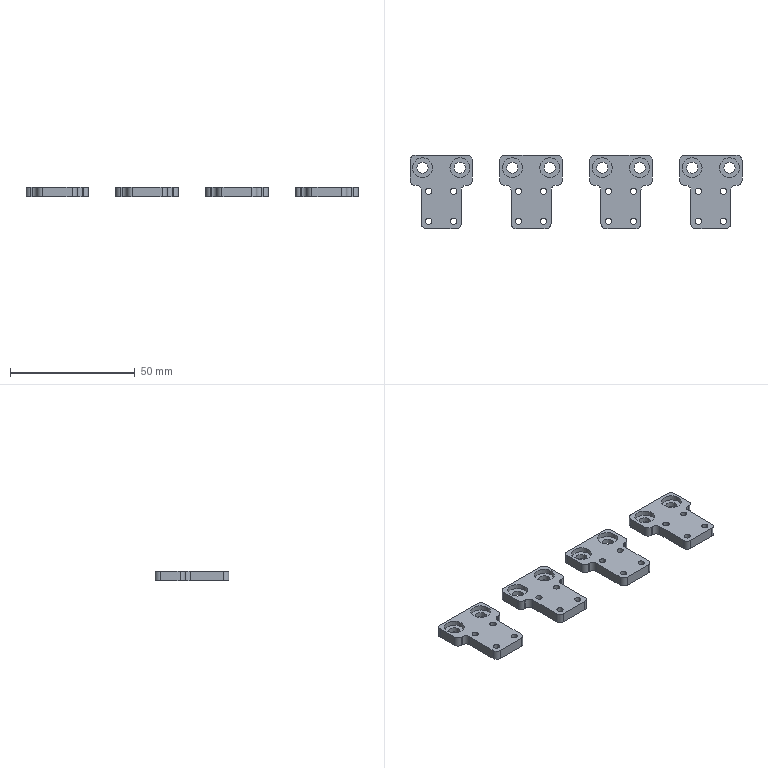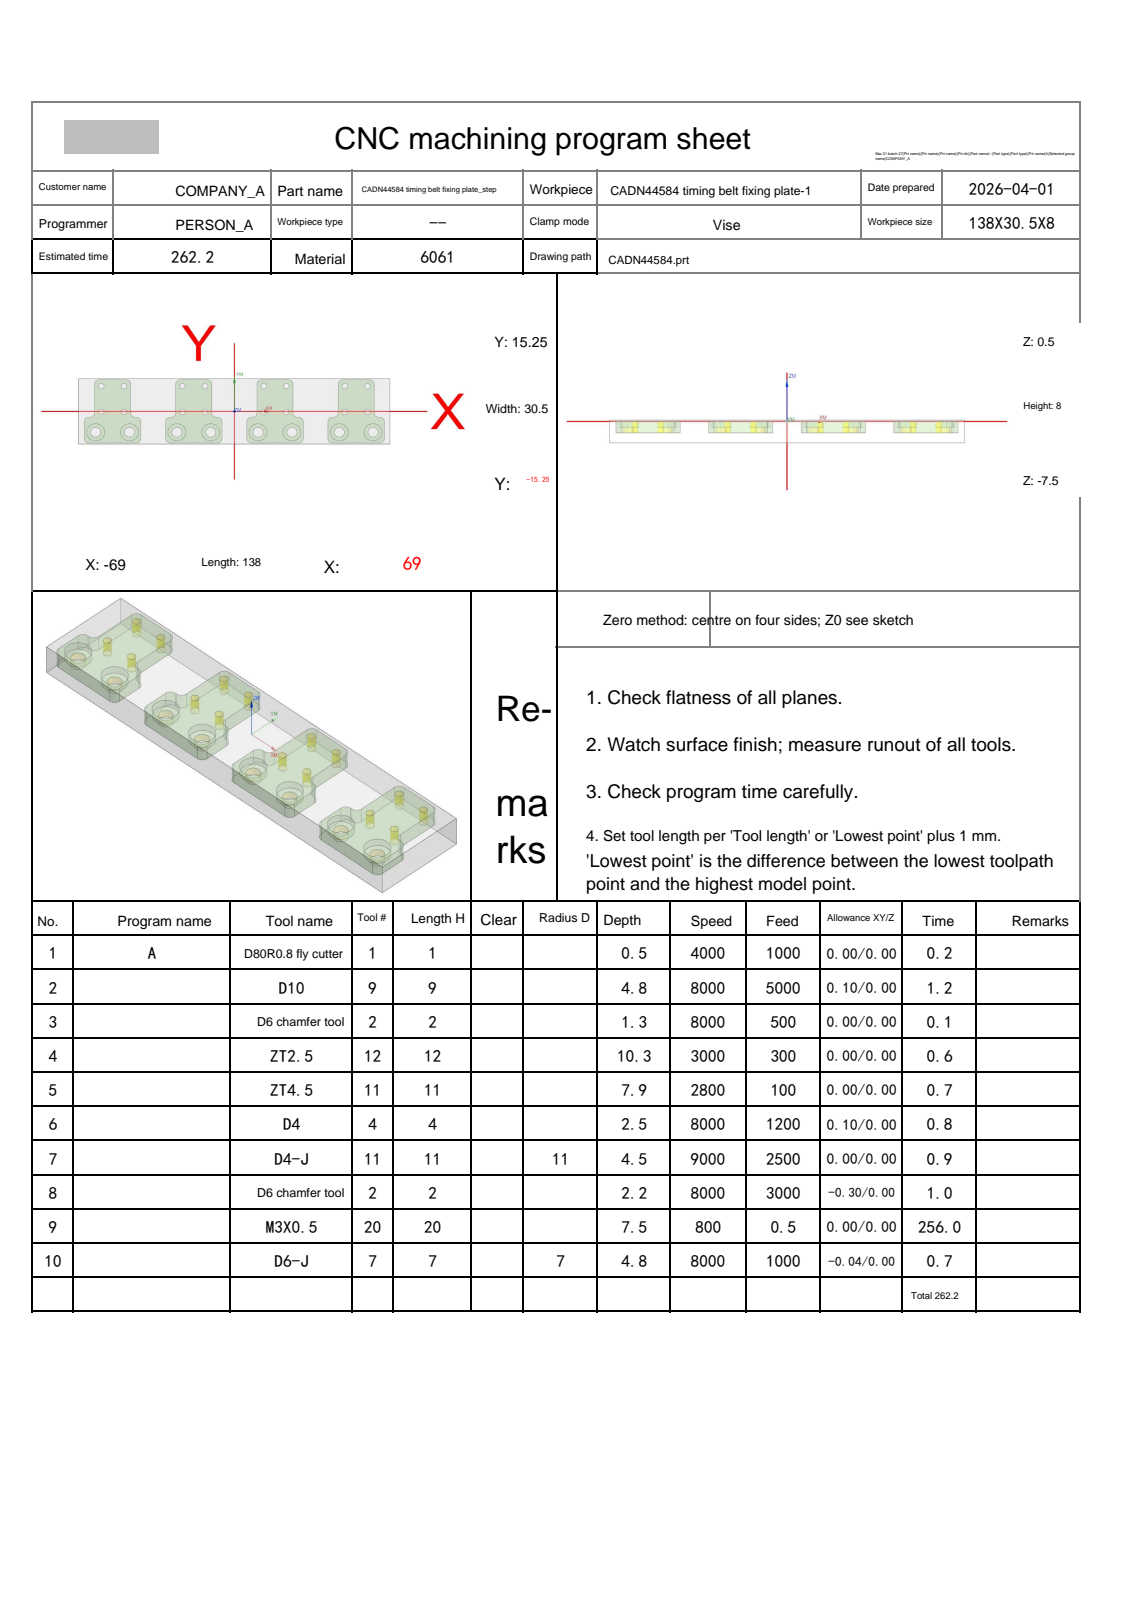NC program | NX | posted by the shop | part box 133 x 29.5 x 4 mm
Lines 869 to 2008 of 5056:
N7 T11 M06
(D4-J  D=4. R=0. H=11 ce=0.00 di=0.00)
G00 G90 G54 X-25.5 Y-9.75 M03 S8000
G43 H11 Z20.
M08
Z.5
G41 D11
G01 X-25.54 Y-9.554 F500.
G03 X-26.51 Y-8.76 I-.97 J-.196
X-27.5 Y-9.75 I0.0 J-.99
X-23.5 Y-9.75 Z-2. I2. J0.0
X-25.5 Y-7.75 I-2. J0.0
X-27.5 Y-9.75 I0.0 J-2.
X-25.5 Y-11.75 I2. J0.0
X-23.5 Y-9.75 I0.0 J2.
X-24.49 Y-8.76 I-.99 J0.0
X-25.46 Y-9.554 I0.0 J-.99
G01 G40 X-25.5 Y-9.75
G00 Z20.
X-46.5
Z.5
G41 D11
G01 X-46.54 Y-9.554
G03 X-47.51 Y-8.76 I-.97 J-.196
X-48.5 Y-9.75 I0.0 J-.99
X-44.5 Y-9.75 Z-2. I2. J0.0
X-46.5 Y-7.75 I-2. J0.0
X-48.5 Y-9.75 I0.0 J-2.
X-46.5 Y-11.75 I2. J0.0
X-44.5 Y-9.75 I0.0 J2.
X-45.49 Y-8.76 I-.99 J0.0
X-46.46 Y-9.554 I0.0 J-.99
G01 G40 X-46.5 Y-9.75
G00 Z20.
X-61.5
Z.5
G41 D11
G01 X-61.54 Y-9.554
G03 X-62.51 Y-8.76 I-.97 J-.196
X-63.5 Y-9.75 I0.0 J-.99
X-59.5 Y-9.75 Z-2. I2. J0.0
X-61.5 Y-7.75 I-2. J0.0
X-63.5 Y-9.75 I0.0 J-2.
X-61.5 Y-11.75 I2. J0.0
X-59.5 Y-9.75 I0.0 J2.
X-60.49 Y-8.76 I-.99 J0.0
X-61.46 Y-9.554 I0.0 J-.99
G01 G40 X-61.5 Y-9.75
G00 Z20.
X-10.5
Z.5
G41 D11
G01 X-10.54 Y-9.554
G03 X-11.51 Y-8.76 I-.97 J-.196
X-12.5 Y-9.75 I0.0 J-.99
X-8.5 Y-9.75 Z-2. I2. J0.0
X-10.5 Y-7.75 I-2. J0.0
X-12.5 Y-9.75 I0.0 J-2.
X-10.5 Y-11.75 I2. J0.0
X-8.5 Y-9.75 I0.0 J2.
X-9.49 Y-8.76 I-.99 J0.0
X-10.46 Y-9.554 I0.0 J-.99
G01 G40 X-10.5 Y-9.75
G00 Z20.
X10.5
Z.5
G41 D11
G01 X10.46 Y-9.554
G03 X9.49 Y-8.76 I-.97 J-.196
X8.5 Y-9.75 I0.0 J-.99
X12.5 Y-9.75 Z-2. I2. J0.0
X10.5 Y-7.75 I-2. J0.0
X8.5 Y-9.75 I0.0 J-2.
X10.5 Y-11.75 I2. J0.0
X12.5 Y-9.75 I0.0 J2.
X11.51 Y-8.76 I-.99 J0.0
X10.54 Y-9.554 I0.0 J-.99
G01 G40 X10.5 Y-9.75
G00 Z20.
X25.5
Z.5
G41 D11
G01 X25.46 Y-9.554
G03 X24.49 Y-8.76 I-.97 J-.196
X23.5 Y-9.75 I0.0 J-.99
X27.5 Y-9.75 Z-2. I2. J0.0
X25.5 Y-7.75 I-2. J0.0
X23.5 Y-9.75 I0.0 J-2.
X25.5 Y-11.75 I2. J0.0
X27.5 Y-9.75 I0.0 J2.
X26.51 Y-8.76 I-.99 J0.0
X25.54 Y-9.554 I0.0 J-.99
G01 G40 X25.5 Y-9.75
G00 Z20.
X46.5
Z.5
G41 D11
G01 X46.46 Y-9.554
G03 X45.49 Y-8.76 I-.97 J-.196
X44.5 Y-9.75 I0.0 J-.99
X48.5 Y-9.75 Z-2. I2. J0.0
X46.5 Y-7.75 I-2. J0.0
X44.5 Y-9.75 I0.0 J-2.
X46.5 Y-11.75 I2. J0.0
X48.5 Y-9.75 I0.0 J2.
X47.51 Y-8.76 I-.99 J0.0
X46.54 Y-9.554 I0.0 J-.99
G01 G40 X46.5 Y-9.75
G00 Z20.
X61.5
Z.5
G41 D11
G01 X61.46 Y-9.554
G03 X60.49 Y-8.76 I-.97 J-.196
X59.5 Y-9.75 I0.0 J-.99
X63.5 Y-9.75 Z-2. I2. J0.0
X61.5 Y-7.75 I-2. J0.0
X59.5 Y-9.75 I0.0 J-2.
X61.5 Y-11.75 I2. J0.0
X63.5 Y-9.75 I0.0 J2.
X62.51 Y-8.76 I-.99 J0.0
X61.54 Y-9.554 I0.0 J-.99
G01 G40 X61.5 Y-9.75
G00 Z20.
G00 G90 X64.602 Y2.341 M03 S9000
Z20.
Z.318
G01 X64.595 Y2.34 Z.232 F2000.
X64.576 Y2.337 Z.154
X64.546 Y2.332 Z.084
X64.508 Y2.324 Z.022
X64.462 Y2.313 Z-.034
X64.411 Y2.299 Z-.083
X64.357 Y2.282 Z-.126
X64.301 Y2.261 Z-.162
X64.245 Y2.237 Z-.193
X64.19 Y2.209 Z-.219
X64.14 Y2.176 Z-.24
X64.094 Y2.139 Z-.256
X64.056 Y2.097 Z-.268
X64.026 Y2.05 Z-.276
X64.007 Y1.999 Z-.281
X64. Y1.941 Z-.282
Y-.75 F2500.
X64.5
G02 X66.148 Y-1.105 I0.0 J-4.
G01 X66.192 Y-1.111 Z-.283
X66.225 Y-1.085 Z-.285
X66.246 Y-1.032 Z-.289
X66.257 Y-.954 Z-.295
X66.258 Y-.855 Z-.301
X66.249 Y-.738 Z-.309
X66.23 Y-.607 Z-.317
X66.203 Y-.465 Z-.327
X66.166 Y-.316 Z-.337
X66.121 Y-.162 Z-.348
X66.069 Y-.008 Z-.359
X65.927 Y.324 Z-.384
X65.75 Y.639 Z-.41
X65.541 Y.936 Z-.436
X65.303 Y1.211 Z-.463
X65.036 Y1.462 Z-.488
X64.907 Y1.567 Z-.499
X64.776 Y1.665 Z-.51
X64.646 Y1.754 Z-.52
X64.519 Y1.832 Z-.529
X64.4 Y1.898 Z-.538
X64.29 Y1.95 Z-.545
X64.194 Y1.986 Z-.552
X64.114 Y2.005 Z-.557
X64.053 Z-.561
X64.014 Y1.984 Z-.563
X64. Y1.941 Z-.564
Y-.75
X64.5
G02 X66.148 Y-1.105 I0.0 J-4.
G01 X66.192 Y-1.111 Z-.565
X66.225 Y-1.085 Z-.568
X66.246 Y-1.032 Z-.572
X66.257 Y-.954 Z-.577
X66.258 Y-.855 Z-.583
X66.249 Y-.738 Z-.591
X66.23 Y-.607 Z-.6
X66.203 Y-.465 Z-.609
X66.166 Y-.316 Z-.619
X66.121 Y-.162 Z-.63
X66.069 Y-.008 Z-.641
X65.927 Y.324 Z-.666
X65.75 Y.639 Z-.692
X65.541 Y.936 Z-.719
X65.303 Y1.211 Z-.745
X65.036 Y1.462 Z-.77
X64.907 Y1.567 Z-.781
X64.776 Y1.665 Z-.792
X64.646 Y1.754 Z-.802
X64.519 Y1.832 Z-.811
X64.4 Y1.898 Z-.82
X64.29 Y1.95 Z-.827
X64.194 Y1.986 Z-.834
X64.114 Y2.005 Z-.839
X64.053 Z-.843
X64.014 Y1.984 Z-.846
X64. Y1.941
Y-.75
X64.5
G02 X66.148 Y-1.105 I0.0 J-4.
G01 X66.192 Y-1.111 Z-.847
X66.225 Y-1.085 Z-.85
X66.246 Y-1.032 Z-.854
X66.257 Y-.954 Z-.859
X66.258 Y-.855 Z-.866
X66.249 Y-.738 Z-.873
X66.23 Y-.607 Z-.882
X66.203 Y-.465 Z-.891
X66.166 Y-.316 Z-.901
X66.121 Y-.162 Z-.912
X66.069 Y-.008 Z-.923
X65.927 Y.324 Z-.948
X65.75 Y.639 Z-.974
X65.541 Y.936 Z-1.001
X65.303 Y1.211 Z-1.027
X65.036 Y1.462 Z-1.052
X64.907 Y1.567 Z-1.063
X64.776 Y1.665 Z-1.074
X64.646 Y1.754 Z-1.084
X64.519 Y1.832 Z-1.093
X64.4 Y1.898 Z-1.102
X64.29 Y1.95 Z-1.109
X64.194 Y1.986 Z-1.116
X64.114 Y2.005 Z-1.121
X64.053 Z-1.125
X64.014 Y1.984 Z-1.128
X64. Y1.941 Z-1.129
Y-.75
X64.5
G02 X66.148 Y-1.105 I0.0 J-4.
G01 X66.192 Y-1.111
X66.225 Y-1.085 Z-1.132
X66.246 Y-1.032 Z-1.136
X66.257 Y-.954 Z-1.141
X66.258 Y-.855 Z-1.148
X66.249 Y-.738 Z-1.155
X66.23 Y-.607 Z-1.164
X66.203 Y-.465 Z-1.173
X66.166 Y-.316 Z-1.183
X66.121 Y-.162 Z-1.194
X66.069 Y-.008 Z-1.205
X65.927 Y.324 Z-1.23
X65.75 Y.639 Z-1.256
X65.541 Y.936 Z-1.283
X65.303 Y1.211 Z-1.309
X65.036 Y1.462 Z-1.334
X64.907 Y1.567 Z-1.345
X64.776 Y1.665 Z-1.356
X64.646 Y1.754 Z-1.366
X64.519 Y1.832 Z-1.375
X64.4 Y1.898 Z-1.384
X64.29 Y1.95 Z-1.392
X64.194 Y1.986 Z-1.398
X64.114 Y2.005 Z-1.403
X64.053 Z-1.407
X64.014 Y1.984 Z-1.41
X64. Y1.941 Z-1.411
Y-.75
X64.5
G02 X66.148 Y-1.105 I0.0 J-4.
G01 X66.192 Y-1.111 Z-1.412
X66.225 Y-1.085 Z-1.414
X66.246 Y-1.032 Z-1.418
X66.257 Y-.954 Z-1.423
X66.258 Y-.855 Z-1.43
X66.249 Y-.738 Z-1.437
X66.23 Y-.607 Z-1.446
X66.203 Y-.465 Z-1.455
X66.166 Y-.316 Z-1.465
X66.121 Y-.162 Z-1.476
X66.069 Y-.008 Z-1.487
X65.927 Y.324 Z-1.512
X65.75 Y.639 Z-1.539
X65.541 Y.936 Z-1.565
X65.303 Y1.211 Z-1.591
X65.036 Y1.462 Z-1.616
X64.907 Y1.567 Z-1.627
X64.776 Y1.665 Z-1.638
X64.646 Y1.754 Z-1.648
X64.519 Y1.832 Z-1.658
X64.4 Y1.898 Z-1.666
X64.29 Y1.95 Z-1.674
X64.194 Y1.986 Z-1.68
X64.114 Y2.005 Z-1.686
X64.053 Z-1.69
X64.014 Y1.984 Z-1.692
X64. Y1.941 Z-1.693
Y-.75
X64.5
G02 X66.148 Y-1.105 I0.0 J-4.
G01 X66.192 Y-1.111 Z-1.694
X66.225 Y-1.085 Z-1.696
X66.246 Y-1.032 Z-1.7
X66.257 Y-.954 Z-1.705
X66.258 Y-.855 Z-1.712
X66.249 Y-.738 Z-1.72
X66.23 Y-.607 Z-1.728
X66.203 Y-.465 Z-1.738
X66.166 Y-.316 Z-1.748
X66.121 Y-.162 Z-1.758
X66.069 Y-.008 Z-1.769
X65.927 Y.324 Z-1.795
X65.75 Y.639 Z-1.821
X65.541 Y.936 Z-1.847
X65.303 Y1.211 Z-1.873
X65.036 Y1.462 Z-1.899
X64.907 Y1.567 Z-1.91
X64.776 Y1.665 Z-1.92
X64.646 Y1.754 Z-1.93
X64.519 Y1.832 Z-1.94
X64.4 Y1.898 Z-1.948
X64.29 Y1.95 Z-1.956
X64.194 Y1.986 Z-1.962
X64.114 Y2.005 Z-1.968
X64.053 Z-1.972
X64.014 Y1.984 Z-1.974
X64. Y1.941 Z-1.975
Y-.75
X64.5
G02 X66.148 Y-1.105 I0.0 J-4.
G01 X66.192 Y-1.111 Z-1.976
X66.225 Y-1.085 Z-1.978
X66.246 Y-1.032 Z-1.982
X66.257 Y-.954 Z-1.988
X66.258 Y-.855 Z-1.994
X66.249 Y-.738 Z-2.002
X66.23 Y-.607 Z-2.01
X66.203 Y-.465 Z-2.02
X66.166 Y-.316 Z-2.03
X66.121 Y-.162 Z-2.04
X66.069 Y-.008 Z-2.051
X65.927 Y.324 Z-2.077
X65.75 Y.639 Z-2.103
X65.541 Y.936 Z-2.129
X65.303 Y1.211 Z-2.155
X65.036 Y1.462 Z-2.181
X64.907 Y1.567 Z-2.192
X64.776 Y1.665 Z-2.202
X64.646 Y1.754 Z-2.212
X64.519 Y1.832 Z-2.222
X64.4 Y1.898 Z-2.23
X64.29 Y1.95 Z-2.238
X64.194 Y1.986 Z-2.245
X64.114 Y2.005 Z-2.25
X64.053 Z-2.254
X64.014 Y1.984 Z-2.256
X64. Y1.941 Z-2.257
Y-.75
X64.5
G02 X66.148 Y-1.105 I0.0 J-4.
G01 X66.192 Y-1.111 Z-2.258
X66.225 Y-1.085 Z-2.26
X66.246 Y-1.032 Z-2.264
X66.257 Y-.954 Z-2.27
X66.258 Y-.855 Z-2.276
X66.249 Y-.738 Z-2.284
X66.23 Y-.607 Z-2.292
X66.203 Y-.465 Z-2.302
X66.166 Y-.316 Z-2.312
X66.121 Y-.162 Z-2.323
X66.069 Y-.008 Z-2.334
X65.927 Y.324 Z-2.359
X65.75 Y.639 Z-2.385
X65.541 Y.936 Z-2.411
X65.303 Y1.211 Z-2.438
X65.036 Y1.462 Z-2.463
X64.907 Y1.567 Z-2.474
X64.776 Y1.665 Z-2.485
X64.646 Y1.754 Z-2.495
X64.519 Y1.832 Z-2.504
X64.4 Y1.898 Z-2.513
X64.29 Y1.95 Z-2.52
X64.194 Y1.986 Z-2.527
X64.114 Y2.005 Z-2.532
X64.053 Z-2.536
X64.014 Y1.984 Z-2.538
X64. Y1.941 Z-2.539
Y-.75
X64.5
G02 X66.148 Y-1.105 I0.0 J-4.
G01 X66.192 Y-1.111 Z-2.54
X66.225 Y-1.085 Z-2.543
X66.246 Y-1.032 Z-2.547
X66.257 Y-.954 Z-2.552
X66.258 Y-.855 Z-2.558
X66.249 Y-.738 Z-2.566
X66.23 Y-.607 Z-2.575
X66.203 Y-.465 Z-2.584
X66.166 Y-.316 Z-2.594
X66.121 Y-.162 Z-2.605
X66.069 Y-.008 Z-2.616
X65.927 Y.324 Z-2.641
X65.75 Y.639 Z-2.667
X65.541 Y.936 Z-2.694
X65.303 Y1.211 Z-2.72
X65.036 Y1.462 Z-2.745
X64.907 Y1.567 Z-2.756
X64.776 Y1.665 Z-2.767
X64.646 Y1.754 Z-2.777
X64.519 Y1.832 Z-2.786
X64.4 Y1.898 Z-2.795
X64.29 Y1.95 Z-2.802
X64.194 Y1.986 Z-2.809
X64.114 Y2.005 Z-2.814
X64.053 Z-2.818
X64.014 Y1.984 Z-2.821
X64. Y1.941
Y-.75
X64.5
G02 X66.148 Y-1.105 I0.0 J-4.
G01 X66.192 Y-1.111 Z-2.822
X66.225 Y-1.085 Z-2.825
X66.246 Y-1.032 Z-2.829
X66.257 Y-.954 Z-2.834
X66.258 Y-.855 Z-2.841
X66.249 Y-.738 Z-2.848
X66.23 Y-.607 Z-2.857
X66.203 Y-.465 Z-2.866
X66.166 Y-.316 Z-2.876
X66.121 Y-.162 Z-2.887
X66.069 Y-.008 Z-2.898
X65.927 Y.324 Z-2.923
X65.75 Y.639 Z-2.949
X65.541 Y.936 Z-2.976
X65.303 Y1.211 Z-3.002
X65.036 Y1.462 Z-3.027
X64.907 Y1.567 Z-3.038
X64.776 Y1.665 Z-3.049
X64.646 Y1.754 Z-3.059
X64.519 Y1.832 Z-3.068
X64.4 Y1.898 Z-3.077
X64.29 Y1.95 Z-3.084
X64.194 Y1.986 Z-3.091
X64.114 Y2.005 Z-3.096
X64.053 Z-3.1
X64.014 Y1.984 Z-3.103
X64. Y1.941 Z-3.104
Y-.75
X64.5
G02 X66.148 Y-1.105 I0.0 J-4.
G01 X66.192 Y-1.111
X66.225 Y-1.085 Z-3.107
X66.246 Y-1.032 Z-3.111
X66.257 Y-.954 Z-3.116
X66.258 Y-.855 Z-3.123
X66.249 Y-.738 Z-3.13
X66.23 Y-.607 Z-3.139
X66.203 Y-.465 Z-3.148
X66.166 Y-.316 Z-3.158
X66.121 Y-.162 Z-3.169
X66.069 Y-.008 Z-3.18
X65.927 Y.324 Z-3.205
X65.75 Y.639 Z-3.231
X65.541 Y.936 Z-3.258
X65.303 Y1.211 Z-3.284
X65.036 Y1.462 Z-3.309
X64.907 Y1.567 Z-3.32
X64.776 Y1.665 Z-3.331
X64.646 Y1.754 Z-3.341
X64.519 Y1.832 Z-3.35
X64.4 Y1.898 Z-3.359
X64.29 Y1.95 Z-3.367
X64.194 Y1.986 Z-3.373
X64.114 Y2.005 Z-3.378
X64.053 Z-3.382
X64.014 Y1.984 Z-3.385
X64. Y1.941 Z-3.386
Y-.75
X64.5
G02 X66.148 Y-1.105 I0.0 J-4.
G01 X66.192 Y-1.111 Z-3.387
X66.225 Y-1.085 Z-3.389
X66.246 Y-1.032 Z-3.393
X66.257 Y-.954 Z-3.398
X66.258 Y-.855 Z-3.405
X66.249 Y-.738 Z-3.412
X66.23 Y-.607 Z-3.421
X66.203 Y-.465 Z-3.43
X66.166 Y-.316 Z-3.44
X66.121 Y-.162 Z-3.451
X66.069 Y-.008 Z-3.462
X65.927 Y.324 Z-3.487
X65.75 Y.639 Z-3.514
X65.541 Y.936 Z-3.54
X65.303 Y1.211 Z-3.566
X65.036 Y1.462 Z-3.591
X64.907 Y1.567 Z-3.602
X64.776 Y1.665 Z-3.613
X64.646 Y1.754 Z-3.623
X64.519 Y1.832 Z-3.633
X64.4 Y1.898 Z-3.641
X64.29 Y1.95 Z-3.649
X64.194 Y1.986 Z-3.655
X64.114 Y2.005 Z-3.661
X64.053 Z-3.665
X64.014 Y1.984 Z-3.667
X64. Y1.941 Z-3.668
Y-.75
X64.5
G02 X66.148 Y-1.105 I0.0 J-4.
G01 X66.192 Y-1.111 Z-3.669
X66.225 Y-1.085 Z-3.671
X66.246 Y-1.032 Z-3.675
X66.257 Y-.954 Z-3.68
X66.258 Y-.855 Z-3.687
X66.249 Y-.738 Z-3.695
X66.23 Y-.607 Z-3.703
X66.203 Y-.465 Z-3.713
X66.166 Y-.316 Z-3.723
X66.121 Y-.162 Z-3.733
X66.069 Y-.008 Z-3.744
X65.927 Y.324 Z-3.77
X65.75 Y.639 Z-3.796
X65.541 Y.936 Z-3.822
X65.303 Y1.211 Z-3.848
X65.036 Y1.462 Z-3.874
X64.907 Y1.567 Z-3.885
X64.776 Y1.665 Z-3.895
X64.646 Y1.754 Z-3.905
X64.519 Y1.832 Z-3.915
X64.4 Y1.898 Z-3.923
X64.29 Y1.95 Z-3.931
X64.194 Y1.986 Z-3.937
X64.114 Y2.005 Z-3.943
X64.053 Z-3.947
X64.014 Y1.984 Z-3.949
X64. Y1.941 Z-3.95
Y-.75
X64.5
G02 X66.148 Y-1.105 I0.0 J-4.
G01 X66.203 Y-1.123 Z-3.949
X66.258 Y-1.127 Z-3.944
X66.313 Y-1.119 Z-3.936
X66.367 Y-1.101 Z-3.924
X66.42 Y-1.074 Z-3.908
X66.47 Y-1.041 Z-3.887
X66.519 Y-1.003 Z-3.861
X66.564 Y-.962 Z-3.83
X66.606 Y-.919 Z-3.793
X66.644 Y-.876 Z-3.751
X66.678 Y-.836 Z-3.702
X66.707 Y-.798 Z-3.646
X66.73 Y-.766 Z-3.584
X66.747 Y-.742 Z-3.514
X66.758 Y-.725 Z-3.436
X66.762 Y-.72 Z-3.35
G00 Z20.
X41.219 Y-.727
Z.318
G01 X41.223 Y-.733 Z.232 F2000.
X41.234 Y-.749 Z.154
X41.252 Y-.774 Z.084
X41.277 Y-.805 Z.022
X41.307 Y-.842 Z-.034
X41.342 Y-.882 Z-.083
X41.382 Y-.924 Z-.126
X41.426 Y-.966 Z-.162
X41.473 Y-1.006 Z-.193
X41.523 Y-1.044 Z-.219
X41.576 Y-1.076 Z-.24
X41.63 Y-1.102 Z-.256
X41.685 Y-1.119 Z-.268
X41.741 Y-1.127 Z-.276
X41.797 Y-1.123 Z-.281
X41.852 Y-1.105 Z-.282
G02 X43.5 Y-.75 I1.648 J-3.645 F2500.
G01 X44.
Y1.941
X43.986 Y1.984 Z-.283
X43.947 Y2.005 Z-.285
X43.886 Z-.289
X43.805 Y1.985 Z-.295
X43.709 Y1.949 Z-.301
X43.599 Y1.897 Z-.309
X43.479 Y1.831 Z-.317
X43.352 Y1.753 Z-.327
X43.221 Y1.664 Z-.337
X43.089 Y1.566 Z-.348
X42.959 Y1.46 Z-.359
X42.691 Y1.209 Z-.384
X42.451 Y.933 Z-.41
X42.241 Y.635 Z-.436
X42.064 Y.32 Z-.463
X41.922 Y-.011 Z-.488
X41.865 Y-.181 Z-.5
X41.819 Y-.349 Z-.512
X41.782 Y-.511 Z-.523
X41.756 Y-.663 Z-.533
X41.742 Y-.8 Z-.542
X41.739 Y-.918 Z-.549
X41.748 Y-1.012 Z-.556
X41.769 Y-1.077 Z-.56
X41.804 Y-1.11 Z-.563
X41.852 Y-1.105 Z-.564
G02 X43.5 Y-.75 I1.648 J-3.645
G01 X44.
Y1.941
X43.986 Y1.984 Z-.565
X43.947 Y2.005 Z-.568
X43.886 Z-.572
X43.805 Y1.985 Z-.577
X43.709 Y1.949 Z-.583
X43.599 Y1.897 Z-.591
X43.479 Y1.831 Z-.6
X43.352 Y1.753 Z-.609
X43.221 Y1.664 Z-.619
X43.089 Y1.566 Z-.63
X42.959 Y1.46 Z-.641
X42.691 Y1.209 Z-.666
X42.451 Y.933 Z-.692
X42.241 Y.635 Z-.719
X42.064 Y.32 Z-.745
X41.922 Y-.011 Z-.77
X41.865 Y-.181 Z-.782
X41.819 Y-.349 Z-.794
X41.782 Y-.511 Z-.805
X41.756 Y-.663 Z-.815
X41.742 Y-.8 Z-.824
X41.739 Y-.918 Z-.831
X41.748 Y-1.012 Z-.838
X41.769 Y-1.077 Z-.842
X41.804 Y-1.11 Z-.845
X41.852 Y-1.105 Z-.846
G02 X43.5 Y-.75 I1.648 J-3.645
G01 X44.
Y1.941
X43.986 Y1.984 Z-.847
X43.947 Y2.005 Z-.85
X43.886 Z-.854
X43.805 Y1.985 Z-.859
X43.709 Y1.949 Z-.866
X43.599 Y1.897 Z-.873
X43.479 Y1.831 Z-.882
X43.352 Y1.753 Z-.891
X43.221 Y1.664 Z-.901
X43.089 Y1.566 Z-.912
X42.959 Y1.46 Z-.923
X42.691 Y1.209 Z-.948
X42.451 Y.933 Z-.974
X42.241 Y.635 Z-1.001
X42.064 Y.32 Z-1.027
X41.922 Y-.011 Z-1.052
X41.865 Y-.181 Z-1.064
X41.819 Y-.349 Z-1.076
X41.782 Y-.511 Z-1.087
X41.756 Y-.663 Z-1.097
X41.742 Y-.8 Z-1.106
X41.739 Y-.918 Z-1.114
X41.748 Y-1.012 Z-1.12
X41.769 Y-1.077 Z-1.125
X41.804 Y-1.11 Z-1.128
X41.852 Y-1.105 Z-1.129
G02 X43.5 Y-.75 I1.648 J-3.645
G01 X44.
Y1.941
X43.986 Y1.984
X43.947 Y2.005 Z-1.132
X43.886 Z-1.136
X43.805 Y1.985 Z-1.141
X43.709 Y1.949 Z-1.148
X43.599 Y1.897 Z-1.155
X43.479 Y1.831 Z-1.164
X43.352 Y1.753 Z-1.173
X43.221 Y1.664 Z-1.183
X43.089 Y1.566 Z-1.194
X42.959 Y1.46 Z-1.205
X42.691 Y1.209 Z-1.23
X42.451 Y.933 Z-1.256
X42.241 Y.635 Z-1.283
X42.064 Y.32 Z-1.309
X41.922 Y-.011 Z-1.334
X41.865 Y-.181 Z-1.346
X41.819 Y-.349 Z-1.358
X41.782 Y-.511 Z-1.369
X41.756 Y-.663 Z-1.379
X41.742 Y-.8 Z-1.388
X41.739 Y-.918 Z-1.396
X41.748 Y-1.012 Z-1.402
X41.769 Y-1.077 Z-1.407
X41.804 Y-1.11 Z-1.41
X41.852 Y-1.105 Z-1.411
G02 X43.5 Y-.75 I1.648 J-3.645
G01 X44.
Y1.941
X43.986 Y1.984 Z-1.412
X43.947 Y2.005 Z-1.414
X43.886 Z-1.418
X43.805 Y1.985 Z-1.423
X43.709 Y1.949 Z-1.43
X43.599 Y1.897 Z-1.437
X43.479 Y1.831 Z-1.446
X43.352 Y1.753 Z-1.455
X43.221 Y1.664 Z-1.465
X43.089 Y1.566 Z-1.476
X42.959 Y1.46 Z-1.487
X42.691 Y1.209 Z-1.512
X42.451 Y.933 Z-1.539
X42.241 Y.635 Z-1.565
X42.064 Y.32 Z-1.591
X41.922 Y-.011 Z-1.616
X41.865 Y-.181 Z-1.629
X41.819 Y-.349 Z-1.64
X41.782 Y-.511 Z-1.651
X41.756 Y-.663 Z-1.661
X41.742 Y-.8 Z-1.67
X41.739 Y-.918 Z-1.678
X41.748 Y-1.012 Z-1.684
X41.769 Y-1.077 Z-1.689
X41.804 Y-1.11 Z-1.692
X41.852 Y-1.105 Z-1.693
G02 X43.5 Y-.75 I1.648 J-3.645
G01 X44.
Y1.941
X43.986 Y1.984 Z-1.694
X43.947 Y2.005 Z-1.696
X43.886 Z-1.7
X43.805 Y1.985 Z-1.705
X43.709 Y1.949 Z-1.712
X43.599 Y1.897 Z-1.72
X43.479 Y1.831 Z-1.728
X43.352 Y1.753 Z-1.738
X43.221 Y1.664 Z-1.748
X43.089 Y1.566 Z-1.758
X42.959 Y1.46 Z-1.769
X42.691 Y1.209 Z-1.795
X42.451 Y.933 Z-1.821
X42.241 Y.635 Z-1.847
X42.064 Y.32 Z-1.873
X41.922 Y-.011 Z-1.899
X41.865 Y-.181 Z-1.911
X41.819 Y-.349 Z-1.922
X41.782 Y-.511 Z-1.933
X41.756 Y-.663 Z-1.943
X41.742 Y-.8 Z-1.952
X41.739 Y-.918 Z-1.96
X41.748 Y-1.012 Z-1.966
X41.769 Y-1.077 Z-1.971
X41.804 Y-1.11 Z-1.974
X41.852 Y-1.105 Z-1.975
G02 X43.5 Y-.75 I1.648 J-3.645
G01 X44.
Y1.941
X43.986 Y1.984 Z-1.976
X43.947 Y2.005 Z-1.978
X43.886 Z-1.982
X43.805 Y1.985 Z-1.988
X43.709 Y1.949 Z-1.994
X43.599 Y1.897 Z-2.002
X43.479 Y1.831 Z-2.01
X43.352 Y1.753 Z-2.02
X43.221 Y1.664 Z-2.03
X43.089 Y1.566 Z-2.04
X42.959 Y1.46 Z-2.051
X42.691 Y1.209 Z-2.077
X42.451 Y.933 Z-2.103
X42.241 Y.635 Z-2.129
X42.064 Y.32 Z-2.155
X41.922 Y-.011 Z-2.181
X41.865 Y-.181 Z-2.193
X41.819 Y-.349 Z-2.204
X41.782 Y-.511 Z-2.215
X41.756 Y-.663 Z-2.225
X41.742 Y-.8 Z-2.234
X41.739 Y-.918 Z-2.242
X41.748 Y-1.012 Z-2.248
X41.769 Y-1.077 Z-2.253
X41.804 Y-1.11 Z-2.256
X41.852 Y-1.105 Z-2.257
G02 X43.5 Y-.75 I1.648 J-3.645
G01 X44.
Y1.941
X43.986 Y1.984 Z-2.258
X43.947 Y2.005 Z-2.26
X43.886 Z-2.264
X43.805 Y1.985 Z-2.27
X43.709 Y1.949 Z-2.276
X43.599 Y1.897 Z-2.284
X43.479 Y1.831 Z-2.292
X43.352 Y1.753 Z-2.302
X43.221 Y1.664 Z-2.312
X43.089 Y1.566 Z-2.323
X42.959 Y1.46 Z-2.334
X42.691 Y1.209 Z-2.359
X42.451 Y.933 Z-2.385
X42.241 Y.635 Z-2.411
X42.064 Y.32 Z-2.438
X41.922 Y-.011 Z-2.463
X41.865 Y-.181 Z-2.475
X41.819 Y-.349 Z-2.487
X41.782 Y-.511 Z-2.498
X41.756 Y-.663 Z-2.508
X41.742 Y-.8 Z-2.517
X41.739 Y-.918 Z-2.524
X41.748 Y-1.012 Z-2.531
X41.769 Y-1.077 Z-2.535
X41.804 Y-1.11 Z-2.538
X41.852 Y-1.105 Z-2.539
G02 X43.5 Y-.75 I1.648 J-3.645
G01 X44.
Y1.941
X43.986 Y1.984 Z-2.54
X43.947 Y2.005 Z-2.543
X43.886 Z-2.547
X43.805 Y1.985 Z-2.552
X43.709 Y1.949 Z-2.558
X43.599 Y1.897 Z-2.566
X43.479 Y1.831 Z-2.575
X43.352 Y1.753 Z-2.584
X43.221 Y1.664 Z-2.594
X43.089 Y1.566 Z-2.605
X42.959 Y1.46 Z-2.616
X42.691 Y1.209 Z-2.641
X42.451 Y.933 Z-2.667
X42.241 Y.635 Z-2.694
X42.064 Y.32 Z-2.72
X41.922 Y-.011 Z-2.745
X41.865 Y-.181 Z-2.757
X41.819 Y-.349 Z-2.769
X41.782 Y-.511 Z-2.78
X41.756 Y-.663 Z-2.79
X41.742 Y-.8 Z-2.799
X41.739 Y-.918 Z-2.806
X41.748 Y-1.012 Z-2.813
X41.769 Y-1.077 Z-2.817
X41.804 Y-1.11 Z-2.82
X41.852 Y-1.105 Z-2.821
G02 X43.5 Y-.75 I1.648 J-3.645
G01 X44.
Y1.941
X43.986 Y1.984 Z-2.822
X43.947 Y2.005 Z-2.825
X43.886 Z-2.829
X43.805 Y1.985 Z-2.834
X43.709 Y1.949 Z-2.841
X43.599 Y1.897 Z-2.848
X43.479 Y1.831 Z-2.857
X43.352 Y1.753 Z-2.866
X43.221 Y1.664 Z-2.876
X43.089 Y1.566 Z-2.887
X42.959 Y1.46 Z-2.898
X42.691 Y1.209 Z-2.923
X42.451 Y.933 Z-2.949
X42.241 Y.635 Z-2.976
X42.064 Y.32 Z-3.002
X41.922 Y-.011 Z-3.027
X41.865 Y-.181 Z-3.039
X41.819 Y-.349 Z-3.051
X41.782 Y-.511 Z-3.062
X41.756 Y-.663 Z-3.072
X41.742 Y-.8 Z-3.081
X41.739 Y-.918 Z-3.089
X41.748 Y-1.012 Z-3.095
X41.769 Y-1.077 Z-3.1
X41.804 Y-1.11 Z-3.103
X41.852 Y-1.105 Z-3.104
G02 X43.5 Y-.75 I1.648 J-3.645
G01 X44.
Y1.941
X43.986 Y1.984
X43.947 Y2.005 Z-3.107
X43.886 Z-3.111
X43.805 Y1.985 Z-3.116
X43.709 Y1.949 Z-3.123
X43.599 Y1.897 Z-3.13
X43.479 Y1.831 Z-3.139
X43.352 Y1.753 Z-3.148
X43.221 Y1.664 Z-3.158
X43.089 Y1.566 Z-3.169
X42.959 Y1.46 Z-3.18
X42.691 Y1.209 Z-3.205
X42.451 Y.933 Z-3.231
X42.241 Y.635 Z-3.258
X42.064 Y.32 Z-3.284
X41.922 Y-.011 Z-3.309
X41.865 Y-.181 Z-3.321
X41.819 Y-.349 Z-3.333
X41.782 Y-.511 Z-3.344
X41.756 Y-.663 Z-3.354
X41.742 Y-.8 Z-3.363
X41.739 Y-.918 Z-3.371
X41.748 Y-1.012 Z-3.377
X41.769 Y-1.077 Z-3.382
X41.804 Y-1.11 Z-3.385
X41.852 Y-1.105 Z-3.386
G02 X43.5 Y-.75 I1.648 J-3.645
G01 X44.
Y1.941
X43.986 Y1.984 Z-3.387
X43.947 Y2.005 Z-3.389
X43.886 Z-3.393
X43.805 Y1.985 Z-3.398
X43.709 Y1.949 Z-3.405
X43.599 Y1.897 Z-3.412
X43.479 Y1.831 Z-3.421
X43.352 Y1.753 Z-3.43
X43.221 Y1.664 Z-3.44
X43.089 Y1.566 Z-3.451
X42.959 Y1.46 Z-3.462
X42.691 Y1.209 Z-3.487
X42.451 Y.933 Z-3.514
X42.241 Y.635 Z-3.54
X42.064 Y.32 Z-3.566
X41.922 Y-.011 Z-3.591
X41.865 Y-.181 Z-3.604
X41.819 Y-.349 Z-3.615
X41.782 Y-.511 Z-3.626
X41.756 Y-.663 Z-3.636
X41.742 Y-.8 Z-3.645
X41.739 Y-.918 Z-3.653
X41.748 Y-1.012 Z-3.659
X41.769 Y-1.077 Z-3.664
X41.804 Y-1.11 Z-3.667
X41.852 Y-1.105 Z-3.668
G02 X43.5 Y-.75 I1.648 J-3.645
G01 X44.
Y1.941
X43.986 Y1.984 Z-3.669
X43.947 Y2.005 Z-3.671
X43.886 Z-3.675
X43.805 Y1.985 Z-3.68
X43.709 Y1.949 Z-3.687
X43.599 Y1.897 Z-3.695
X43.479 Y1.831 Z-3.703
X43.352 Y1.753 Z-3.713
X43.221 Y1.664 Z-3.723
X43.089 Y1.566 Z-3.733
X42.959 Y1.46 Z-3.744
X42.691 Y1.209 Z-3.77
X42.451 Y.933 Z-3.796
X42.241 Y.635 Z-3.822
X42.064 Y.32 Z-3.848
X41.922 Y-.011 Z-3.874
X41.865 Y-.181 Z-3.886
X41.819 Y-.349 Z-3.897
X41.782 Y-.511 Z-3.908
X41.756 Y-.663 Z-3.918
X41.742 Y-.8 Z-3.927
X41.739 Y-.918 Z-3.935
X41.748 Y-1.012 Z-3.941
X41.769 Y-1.077 Z-3.946
X41.804 Y-1.11 Z-3.949
X41.852 Y-1.105 Z-3.95
G02 X43.5 Y-.75 I1.648 J-3.645
G01 X44.
Y1.941
X43.993 Y1.999 Z-3.949
X43.974 Y2.05 Z-3.944
X43.945 Y2.097 Z-3.936
X43.906 Y2.139 Z-3.924
X43.861 Y2.176 Z-3.908
X43.81 Y2.209 Z-3.887
X43.756 Y2.237 Z-3.861
X43.7 Y2.261 Z-3.83
X43.644 Y2.282 Z-3.793
X43.59 Y2.299 Z-3.751
X43.539 Y2.313 Z-3.702
X43.494 Y2.324 Z-3.646
X43.455 Y2.332 Z-3.584
X43.426 Y2.337 Z-3.514
X43.407 Y2.34 Z-3.436
X43.4 Y2.341 Z-3.35
G00 Z20.
X5.24 Y-.723
Z.318
G01 X5.244 Y-.729 Z.232 F2000.
X5.254 Y-.745 Z.154
X5.272 Y-.77 Z.084
X5.295 Y-.802 Z.022
X5.323 Y-.839 Z-.034
X5.357 Y-.879 Z-.083
X5.395 Y-.921 Z-.126
X5.437 Y-.964 Z-.162
X5.482 Y-1.005 Z-.193
X5.53 Y-1.042 Z-.219
X5.581 Y-1.075 Z-.24
X5.633 Y-1.101 Z-.256
X5.687 Y-1.119 Z-.268
X5.742 Y-1.127 Z-.276
X5.797 Y-1.123 Z-.281
X5.852 Y-1.105 Z-.282
G02 X7.5 Y-.75 I1.648 J-3.645 F2500.
G01 X8.
Y1.941
X7.986 Y1.984 Z-.283
X7.948 Y2.005 Z-.285
X7.887 Z-.289
X7.806 Y1.986 Z-.295
X7.71 Y1.949 Z-.301
X7.601 Y1.897 Z-.309
X7.481 Y1.831 Z-.317
X7.355 Y1.753 Z-.327
X7.225 Y1.664 Z-.337
X7.094 Y1.566 Z-.348
X6.965 Y1.461 Z-.359
X6.699 Y1.21 Z-.384
X6.46 Y.934 Z-.41
X6.252 Y.637 Z-.436
X6.075 Y.322 Z-.463
X5.932 Y-.009 Z-.488
X5.88 Y-.164 Z-.499
X5.835 Y-.317 Z-.51
X5.798 Y-.467 Z-.52
X5.77 Y-.608 Z-.529
X5.752 Y-.739 Z-.538
X5.743 Y-.856 Z-.545
Y-.955 Z-.552
X5.754 Y-1.032 Z-.557
X5.775 Y-1.086 Z-.561
X5.808 Y-1.111 Z-.563
X5.852 Y-1.105 Z-.564
G02 X7.5 Y-.75 I1.648 J-3.645
G01 X8.
Y1.941
X7.986 Y1.984 Z-.565
X7.948 Y2.005 Z-.568
X7.887 Z-.572
X7.806 Y1.986 Z-.577
X7.71 Y1.949 Z-.583
X7.601 Y1.897 Z-.591
X7.481 Y1.831 Z-.6
X7.355 Y1.753 Z-.609
X7.225 Y1.664 Z-.619
X7.094 Y1.566 Z-.63
X6.965 Y1.461 Z-.641
X6.699 Y1.21 Z-.666
X6.46 Y.934 Z-.692
X6.252 Y.637 Z-.719
X6.075 Y.322 Z-.745
X5.932 Y-.009 Z-.77
X5.88 Y-.164 Z-.781
X5.835 Y-.317 Z-.792
X5.798 Y-.467 Z-.802
X5.77 Y-.608 Z-.811
X5.752 Y-.739 Z-.82
X5.743 Y-.856 Z-.827
Y-.955 Z-.834
X5.754 Y-1.032 Z-.839
X5.775 Y-1.086 Z-.843
X5.808 Y-1.111 Z-.846
X5.852 Y-1.105
G02 X7.5 Y-.75 I1.648 J-3.645
G01 X8.
Y1.941
X7.986 Y1.984 Z-.847
X7.948 Y2.005 Z-.85
X7.887 Z-.854
X7.806 Y1.986 Z-.859
X7.71 Y1.949 Z-.866
X7.601 Y1.897 Z-.873
X7.481 Y1.831 Z-.882
X7.355 Y1.753 Z-.891
X7.225 Y1.664 Z-.901
X7.094 Y1.566 Z-.912
X6.965 Y1.461 Z-.923
X6.699 Y1.21 Z-.948
X6.46 Y.934 Z-.974
X6.252 Y.637 Z-1.001
X6.075 Y.322 Z-1.027
X5.932 Y-.009 Z-1.052
X5.88 Y-.164 Z-1.063
X5.835 Y-.317 Z-1.074
X5.798 Y-.467 Z-1.084
X5.77 Y-.608 Z-1.093
X5.752 Y-.739 Z-1.102
X5.743 Y-.856 Z-1.109
Y-.955 Z-1.116
X5.754 Y-1.032 Z-1.121
X5.775 Y-1.086 Z-1.125
X5.808 Y-1.111 Z-1.128
X5.852 Y-1.105 Z-1.129
G02 X7.5 Y-.75 I1.648 J-3.645
G01 X8.
Y1.941
X7.986 Y1.984
X7.948 Y2.005 Z-1.132
X7.887 Z-1.136
X7.806 Y1.986 Z-1.141
X7.71 Y1.949 Z-1.148
X7.601 Y1.897 Z-1.155
X7.481 Y1.831 Z-1.164
X7.355 Y1.753 Z-1.173
X7.225 Y1.664 Z-1.183
X7.094 Y1.566 Z-1.194
X6.965 Y1.461 Z-1.205
X6.699 Y1.21 Z-1.23
X6.46 Y.934 Z-1.256
X6.252 Y.637 Z-1.283
X6.075 Y.322 Z-1.309
X5.932 Y-.009 Z-1.334
X5.88 Y-.164 Z-1.345
X5.835 Y-.317 Z-1.356
X5.798 Y-.467 Z-1.366
X5.77 Y-.608 Z-1.375
X5.752 Y-.739 Z-1.384
X5.743 Y-.856 Z-1.392
Y-.955 Z-1.398
X5.754 Y-1.032 Z-1.403
X5.775 Y-1.086 Z-1.407
X5.808 Y-1.111 Z-1.41
X5.852 Y-1.105 Z-1.411
G02 X7.5 Y-.75 I1.648 J-3.645
G01 X8.
Y1.941
X7.986 Y1.984 Z-1.412
X7.948 Y2.005 Z-1.414
X7.887 Z-1.418
X7.806 Y1.986 Z-1.423
X7.71 Y1.949 Z-1.43
X7.601 Y1.897 Z-1.437
X7.481 Y1.831 Z-1.446
X7.355 Y1.753 Z-1.455
X7.225 Y1.664 Z-1.465
X7.094 Y1.566 Z-1.476
X6.965 Y1.461 Z-1.487
X6.699 Y1.21 Z-1.512
X6.46 Y.934 Z-1.539
X6.252 Y.637 Z-1.565
X6.075 Y.322 Z-1.591
X5.932 Y-.009 Z-1.616
X5.88 Y-.164 Z-1.627
X5.835 Y-.317 Z-1.638
X5.798 Y-.467 Z-1.648
X5.77 Y-.608 Z-1.658
X5.752 Y-.739 Z-1.666
X5.743 Y-.856 Z-1.674
Y-.955 Z-1.68
X5.754 Y-1.032 Z-1.686
X5.775 Y-1.086 Z-1.69
X5.808 Y-1.111 Z-1.692
X5.852 Y-1.105 Z-1.693
G02 X7.5 Y-.75 I1.648 J-3.645
G01 X8.
Y1.941
X7.986 Y1.984 Z-1.694